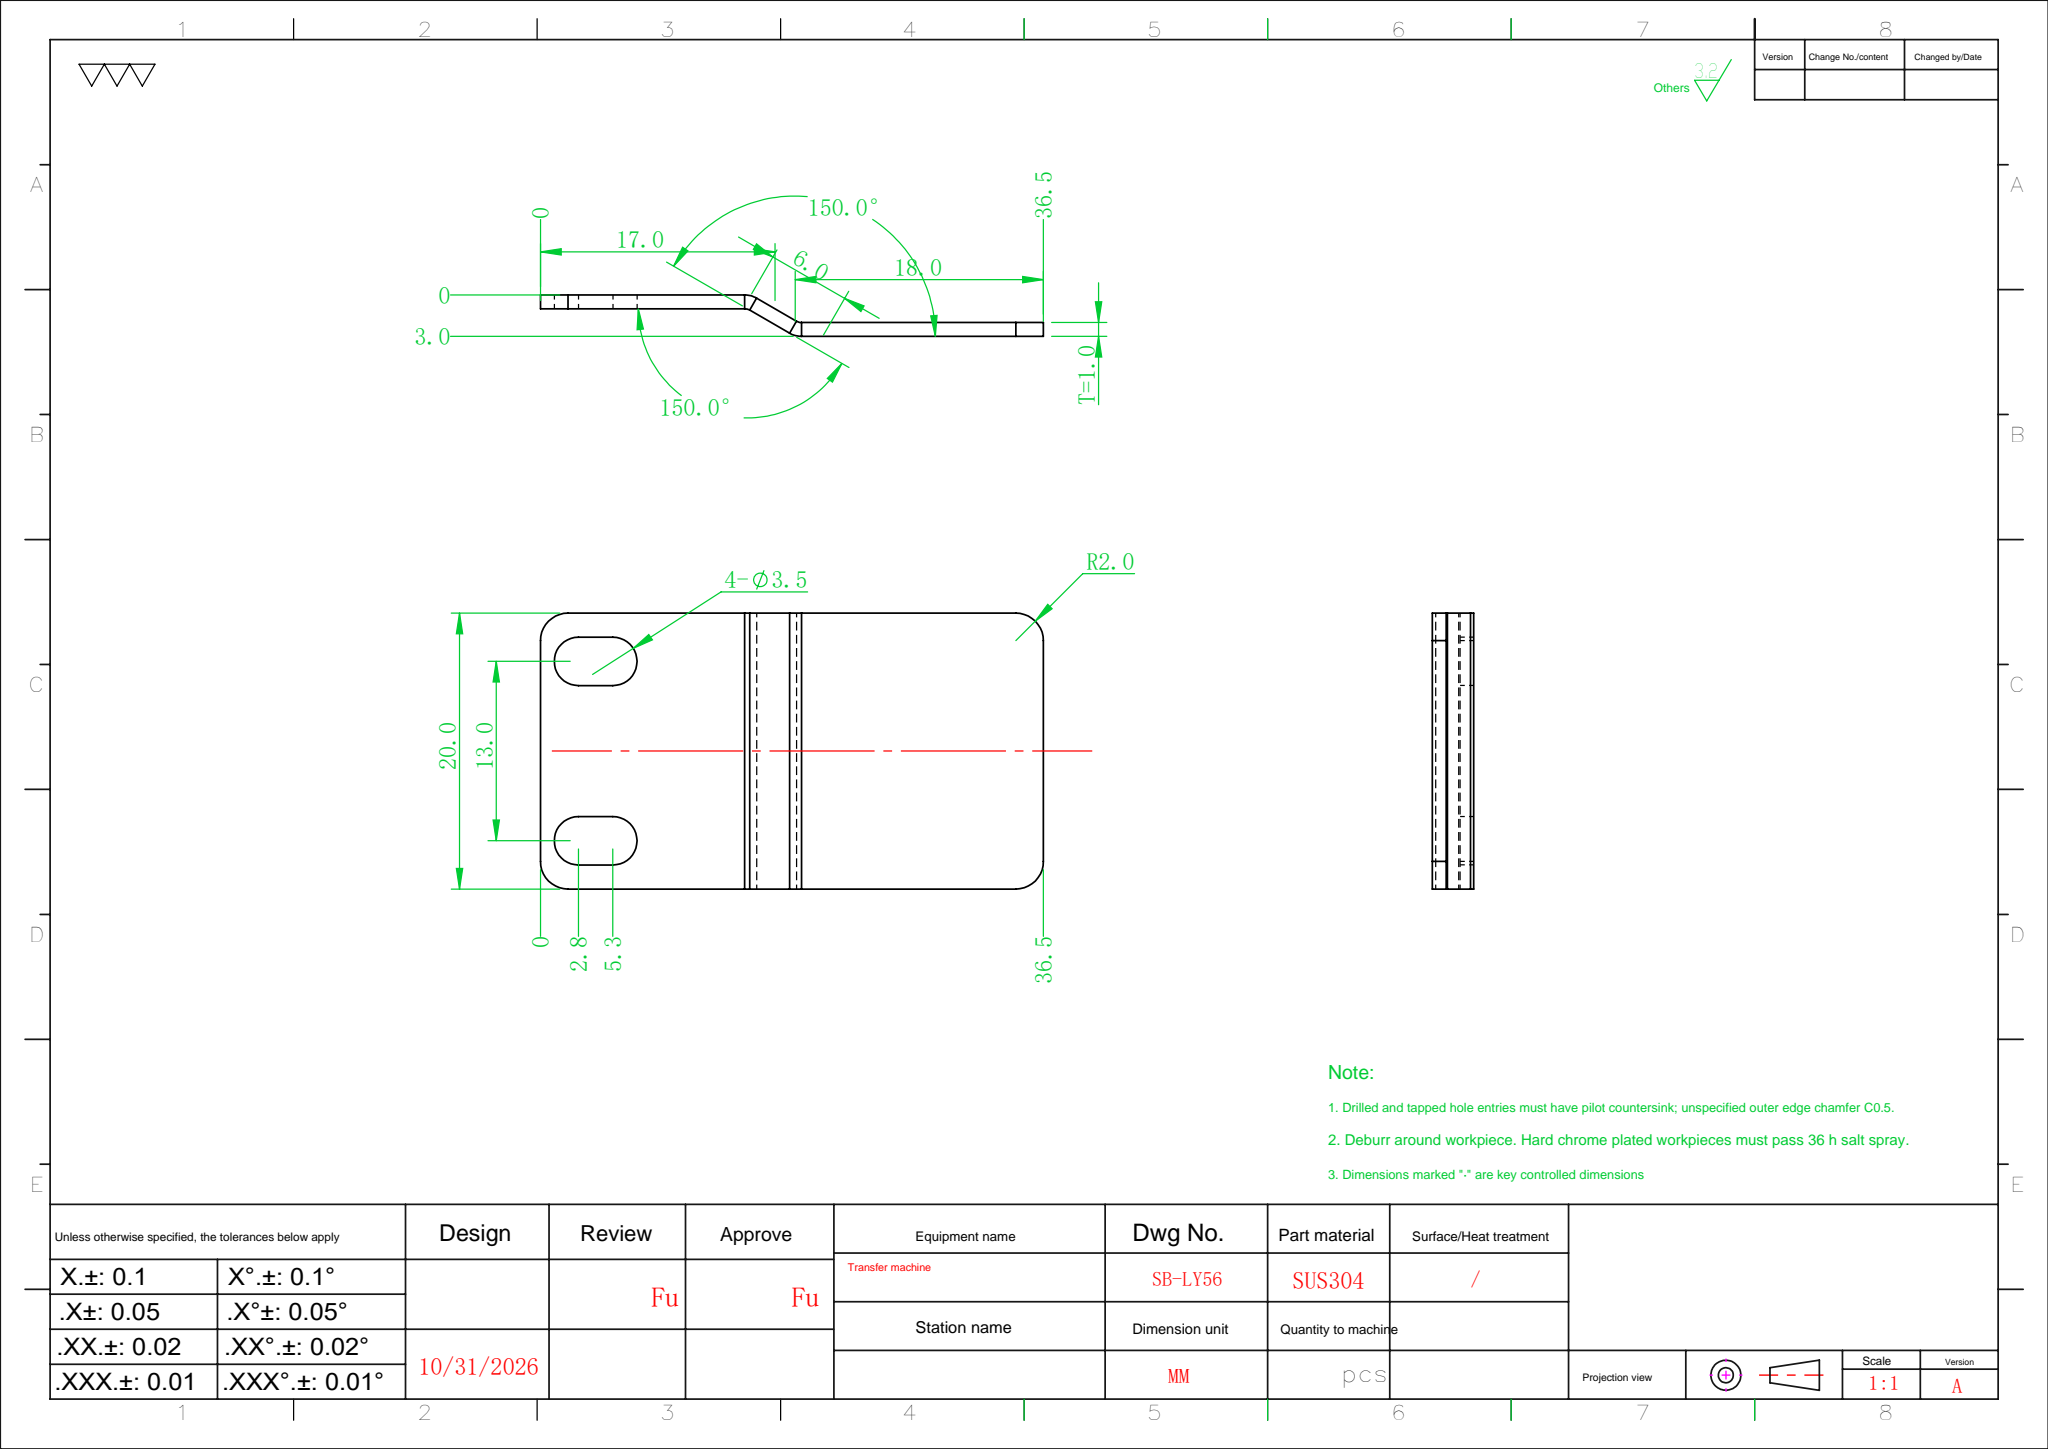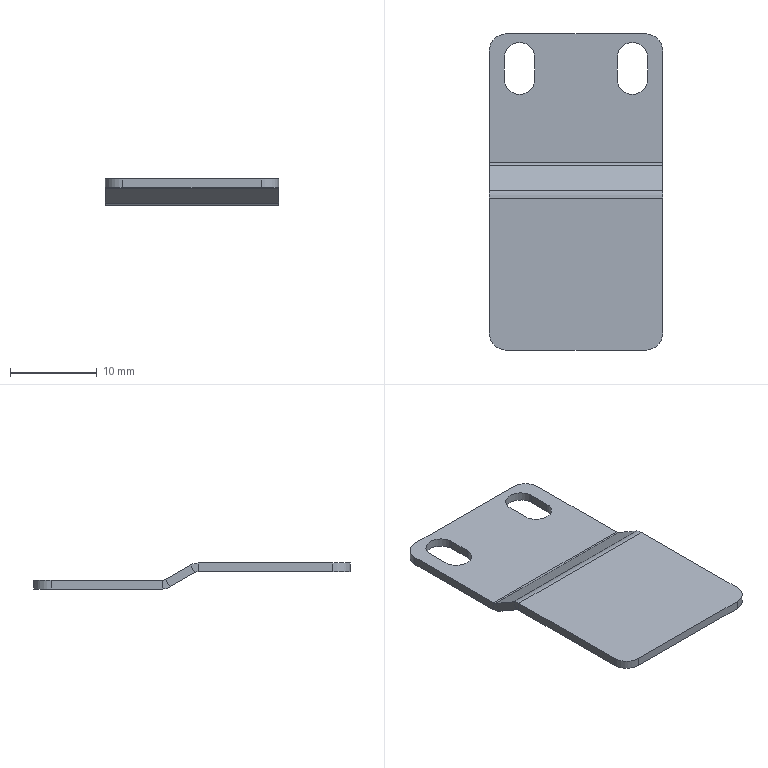Part | SolidWorks | features EdgeFlange 2, Fillet 1, FlatPattern 1, HoleWzd 1, SMBaseFlange 1, SheetMetal 1 | 1 solid | 34 faces | box 20 x 36.464 x 3 mm | volume 699.216 mm3 | plane 22 | cylinder 12 | commonest cylinder face diameters 3.5 x4 4 x4 1.473 x2 3.473 x2
STEP:
#1=CARTESIAN_POINT('',(-10.,-10.061,0.9013));
#2=VERTEX_POINT('',#1);
#3=CARTESIAN_POINT('',(-10.,-9.561,1.767));
#4=VERTEX_POINT('',#3);
#5=CARTESIAN_POINT('',(-10.,-10.061,0.9013));
#6=DIRECTION('',(0.,0.5,0.866));
#7=VECTOR('',#6,1000.);
#8=LINE('',#5,#7);
#9=EDGE_CURVE('',#2,#4,#8,.T.);
#10=ORIENTED_EDGE('',*,*,#9,.T.);
#11=CARTESIAN_POINT('',(-10.,-6.671,0.09869));
#12=VERTEX_POINT('',#11);
#13=CARTESIAN_POINT('',(-10.,-6.5,0.));
#14=DIRECTION('',(0.,0.866,-0.5));
#15=VECTOR('',#14,1000.);
#16=LINE('',#13,#15);
#17=EDGE_CURVE('',#4,#12,#16,.T.);
#18=ORIENTED_EDGE('',*,*,#17,.T.);
#19=CARTESIAN_POINT('',(-10.,-7.171,-0.7673));
#20=VERTEX_POINT('',#19);
#21=CARTESIAN_POINT('',(-10.,-7.171,-0.7673));
#22=DIRECTION('',(0.,-0.5,-0.866));
#23=VECTOR('',#22,1000.);
#24=LINE('',#21,#23);
#25=EDGE_CURVE('',#12,#20,#24,.T.);
#26=ORIENTED_EDGE('',*,*,#25,.T.);
#27=CARTESIAN_POINT('',(-10.,-0.625,-4.547));
#28=DIRECTION('',(0.,0.866,-0.5));
#29=VECTOR('',#28,1000.);
#30=LINE('',#27,#29);
#31=EDGE_CURVE('',#2,#20,#30,.T.);
#32=ORIENTED_EDGE('',*,*,#31,.F.);
#33=EDGE_LOOP('',(#10,#18,#26,#32));
#34=FACE_OUTER_BOUND('',#33,.T.);
#35=CARTESIAN_POINT('',(-10.,-7.,-0.866));
#36=DIRECTION('',(1.,0.,0.));
#37=DIRECTION('',(0.,1.,0.));
#38=AXIS2_PLACEMENT_3D('',#35,#36,#37);
#39=PLANE('',#38);
#40=ADVANCED_FACE('',(#34),#39,.F.);
#41=CARTESIAN_POINT('',(10.,-10.061,0.9013));
#42=VERTEX_POINT('',#41);
#43=CARTESIAN_POINT('',(10.,-9.561,1.767));
#44=VERTEX_POINT('',#43);
#45=CARTESIAN_POINT('',(10.,-10.061,0.9013));
#46=DIRECTION('',(0.,0.5,0.866));
#47=VECTOR('',#46,1000.);
#48=LINE('',#45,#47);
#49=EDGE_CURVE('',#42,#44,#48,.T.);
#50=ORIENTED_EDGE('',*,*,#49,.F.);
#51=CARTESIAN_POINT('',(10.,-7.171,-0.7673));
#52=VERTEX_POINT('',#51);
#53=CARTESIAN_POINT('',(10.,-0.625,-4.547));
#54=DIRECTION('',(0.,-0.866,0.5));
#55=VECTOR('',#54,1000.);
#56=LINE('',#53,#55);
#57=EDGE_CURVE('',#52,#42,#56,.T.);
#58=ORIENTED_EDGE('',*,*,#57,.F.);
#59=CARTESIAN_POINT('',(10.,-6.671,0.09869));
#60=VERTEX_POINT('',#59);
#61=CARTESIAN_POINT('',(10.,-6.671,0.09869));
#62=DIRECTION('',(0.,-0.5,-0.866));
#63=VECTOR('',#62,1000.);
#64=LINE('',#61,#63);
#65=EDGE_CURVE('',#60,#52,#64,.T.);
#66=ORIENTED_EDGE('',*,*,#65,.F.);
#67=CARTESIAN_POINT('',(10.,-11.464,2.866));
#68=DIRECTION('',(0.,-0.866,0.5));
#69=VECTOR('',#68,1000.);
#70=LINE('',#67,#69);
#71=EDGE_CURVE('',#60,#44,#70,.T.);
#72=ORIENTED_EDGE('',*,*,#71,.T.);
#73=EDGE_LOOP('',(#50,#58,#66,#72));
#74=FACE_OUTER_BOUND('',#73,.T.);
#75=CARTESIAN_POINT('',(10.,-11.964,2.));
#76=DIRECTION('',(-1.,0.,0.));
#77=DIRECTION('',(0.,-1.,0.));
#78=AXIS2_PLACEMENT_3D('',#75,#76,#77);
#79=PLANE('',#78);
#80=ADVANCED_FACE('',(#74),#79,.F.);
#81=CARTESIAN_POINT('',(-10.,-10.061,0.9013));
#82=DIRECTION('',(1.,0.,0.));
#83=VECTOR('',#82,1000.);
#84=LINE('',#81,#83);
#85=EDGE_CURVE('',#2,#42,#84,.T.);
#86=ORIENTED_EDGE('',*,*,#85,.F.);
#87=ORIENTED_EDGE('',*,*,#31,.T.);
#88=CARTESIAN_POINT('',(-10.,-7.171,-0.7673));
#89=DIRECTION('',(-1.,0.,0.));
#90=VECTOR('',#89,1000.);
#91=LINE('',#88,#90);
#92=EDGE_CURVE('',#52,#20,#91,.T.);
#93=ORIENTED_EDGE('',*,*,#92,.F.);
#94=ORIENTED_EDGE('',*,*,#57,.T.);
#95=EDGE_LOOP('',(#86,#87,#93,#94));
#96=FACE_OUTER_BOUND('',#95,.T.);
#97=CARTESIAN_POINT('',(0.,-0.625,-4.547));
#98=DIRECTION('',(0.,0.5,0.866));
#99=DIRECTION('',(0.,-0.866,0.5));
#100=AXIS2_PLACEMENT_3D('',#97,#98,#99);
#101=PLANE('',#100);
#102=ADVANCED_FACE('',(#96),#101,.F.);
#103=ORIENTED_EDGE('',*,*,#17,.F.);
#104=CARTESIAN_POINT('',(-10.,-9.561,1.767));
#105=DIRECTION('',(1.,0.,0.));
#106=VECTOR('',#105,1000.);
#107=LINE('',#104,#106);
#108=EDGE_CURVE('',#4,#44,#107,.T.);
#109=ORIENTED_EDGE('',*,*,#108,.T.);
#110=ORIENTED_EDGE('',*,*,#71,.F.);
#111=CARTESIAN_POINT('',(-10.,-6.671,0.09869));
#112=DIRECTION('',(1.,0.,0.));
#113=VECTOR('',#112,1000.);
#114=LINE('',#111,#113);
#115=EDGE_CURVE('',#12,#60,#114,.T.);
#116=ORIENTED_EDGE('',*,*,#115,.F.);
#117=EDGE_LOOP('',(#103,#109,#110,#116));
#118=FACE_OUTER_BOUND('',#117,.T.);
#119=CARTESIAN_POINT('',(0.,-0.125,-3.681));
#120=DIRECTION('',(0.,0.5,0.866));
#121=DIRECTION('',(0.,-0.866,0.5));
#122=AXIS2_PLACEMENT_3D('',#119,#120,#121);
#123=PLANE('',#122);
#124=ADVANCED_FACE('',(#118),#123,.T.);
#125=CARTESIAN_POINT('',(-4.75,5.75,0.));
#126=VERTEX_POINT('',#125);
#127=CARTESIAN_POINT('',(-8.25,5.75,0.));
#128=VERTEX_POINT('',#127);
#129=CARTESIAN_POINT('',(-6.5,5.75,0.));
#130=DIRECTION('',(0.,0.,1.));
#131=DIRECTION('',(1.,0.,0.));
#132=AXIS2_PLACEMENT_3D('',#129,#130,#131);
#133=CIRCLE('',#132,1.75);
#134=EDGE_CURVE('',#126,#128,#133,.T.);
#135=ORIENTED_EDGE('',*,*,#134,.F.);
#136=CARTESIAN_POINT('',(-4.75,3.25,0.));
#137=VERTEX_POINT('',#136);
#138=CARTESIAN_POINT('',(-4.75,3.25,0.));
#139=DIRECTION('',(0.,1.,0.));
#140=VECTOR('',#139,1000.);
#141=LINE('',#138,#140);
#142=EDGE_CURVE('',#137,#126,#141,.T.);
#143=ORIENTED_EDGE('',*,*,#142,.F.);
#144=CARTESIAN_POINT('',(-8.25,3.25,0.));
#145=VERTEX_POINT('',#144);
#146=CARTESIAN_POINT('',(-6.5,3.25,0.));
#147=DIRECTION('',(0.,0.,1.));
#148=DIRECTION('',(1.,0.,0.));
#149=AXIS2_PLACEMENT_3D('',#146,#147,#148);
#150=CIRCLE('',#149,1.75);
#151=EDGE_CURVE('',#145,#137,#150,.T.);
#152=ORIENTED_EDGE('',*,*,#151,.F.);
#153=CARTESIAN_POINT('',(-8.25,3.25,0.));
#154=DIRECTION('',(0.,1.,0.));
#155=VECTOR('',#154,1000.);
#156=LINE('',#153,#155);
#157=EDGE_CURVE('',#145,#128,#156,.T.);
#158=ORIENTED_EDGE('',*,*,#157,.T.);
#159=EDGE_LOOP('',(#135,#143,#152,#158));
#160=FACE_BOUND('',#159,.T.);
#161=CARTESIAN_POINT('',(8.25,5.75,0.));
#162=VERTEX_POINT('',#161);
#163=CARTESIAN_POINT('',(4.75,5.75,0.));
#164=VERTEX_POINT('',#163);
#165=CARTESIAN_POINT('',(6.5,5.75,0.));
#166=DIRECTION('',(0.,0.,1.));
#167=DIRECTION('',(1.,0.,0.));
#168=AXIS2_PLACEMENT_3D('',#165,#166,#167);
#169=CIRCLE('',#168,1.75);
#170=EDGE_CURVE('',#162,#164,#169,.T.);
#171=ORIENTED_EDGE('',*,*,#170,.F.);
#172=CARTESIAN_POINT('',(8.25,3.25,0.));
#173=VERTEX_POINT('',#172);
#174=CARTESIAN_POINT('',(8.25,3.25,0.));
#175=DIRECTION('',(0.,1.,0.));
#176=VECTOR('',#175,1000.);
#177=LINE('',#174,#176);
#178=EDGE_CURVE('',#173,#162,#177,.T.);
#179=ORIENTED_EDGE('',*,*,#178,.F.);
#180=CARTESIAN_POINT('',(4.75,3.25,0.));
#181=VERTEX_POINT('',#180);
#182=CARTESIAN_POINT('',(6.5,3.25,0.));
#183=DIRECTION('',(0.,0.,1.));
#184=DIRECTION('',(1.,0.,0.));
#185=AXIS2_PLACEMENT_3D('',#182,#183,#184);
#186=CIRCLE('',#185,1.75);
#187=EDGE_CURVE('',#181,#173,#186,.T.);
#188=ORIENTED_EDGE('',*,*,#187,.F.);
#189=CARTESIAN_POINT('',(4.75,3.25,0.));
#190=DIRECTION('',(0.,1.,0.));
#191=VECTOR('',#190,1000.);
#192=LINE('',#189,#191);
#193=EDGE_CURVE('',#181,#164,#192,.T.);
#194=ORIENTED_EDGE('',*,*,#193,.T.);
#195=EDGE_LOOP('',(#171,#179,#188,#194));
#196=FACE_BOUND('',#195,.T.);
#197=CARTESIAN_POINT('',(10.,-6.303,0.));
#198=VERTEX_POINT('',#197);
#199=CARTESIAN_POINT('',(10.,6.5,0.));
#200=VERTEX_POINT('',#199);
#201=CARTESIAN_POINT('',(10.,-8.5,0.));
#202=DIRECTION('',(0.,1.,0.));
#203=VECTOR('',#202,1000.);
#204=LINE('',#201,#203);
#205=EDGE_CURVE('',#198,#200,#204,.T.);
#206=ORIENTED_EDGE('',*,*,#205,.T.);
#207=CARTESIAN_POINT('',(8.,8.5,0.));
#208=VERTEX_POINT('',#207);
#209=CARTESIAN_POINT('',(8.,6.5,0.));
#210=DIRECTION('',(0.,0.,1.));
#211=DIRECTION('',(-1.,0.,0.));
#212=AXIS2_PLACEMENT_3D('',#209,#210,#211);
#213=CIRCLE('',#212,2.);
#214=EDGE_CURVE('',#200,#208,#213,.T.);
#215=ORIENTED_EDGE('',*,*,#214,.T.);
#216=CARTESIAN_POINT('',(-8.,8.5,0.));
#217=VERTEX_POINT('',#216);
#218=CARTESIAN_POINT('',(-10.,8.5,0.));
#219=DIRECTION('',(-1.,0.,0.));
#220=VECTOR('',#219,1000.);
#221=LINE('',#218,#220);
#222=EDGE_CURVE('',#208,#217,#221,.T.);
#223=ORIENTED_EDGE('',*,*,#222,.T.);
#224=CARTESIAN_POINT('',(-10.,6.5,0.));
#225=VERTEX_POINT('',#224);
#226=CARTESIAN_POINT('',(-8.,6.5,0.));
#227=DIRECTION('',(0.,0.,1.));
#228=DIRECTION('',(-1.,0.,0.));
#229=AXIS2_PLACEMENT_3D('',#226,#227,#228);
#230=CIRCLE('',#229,2.);
#231=EDGE_CURVE('',#217,#225,#230,.T.);
#232=ORIENTED_EDGE('',*,*,#231,.T.);
#233=CARTESIAN_POINT('',(-10.,-6.303,0.));
#234=VERTEX_POINT('',#233);
#235=CARTESIAN_POINT('',(-10.,-8.5,0.));
#236=DIRECTION('',(0.,-1.,0.));
#237=VECTOR('',#236,1000.);
#238=LINE('',#235,#237);
#239=EDGE_CURVE('',#225,#234,#238,.T.);
#240=ORIENTED_EDGE('',*,*,#239,.T.);
#241=CARTESIAN_POINT('',(10.,-6.303,0.));
#242=DIRECTION('',(-1.,0.,0.));
#243=VECTOR('',#242,1000.);
#244=LINE('',#241,#243);
#245=EDGE_CURVE('',#198,#234,#244,.T.);
#246=ORIENTED_EDGE('',*,*,#245,.F.);
#247=EDGE_LOOP('',(#206,#215,#223,#232,#240,#246));
#248=FACE_OUTER_BOUND('',#247,.T.);
#249=CARTESIAN_POINT('',(0.,0.,0.));
#250=DIRECTION('',(0.,0.,-1.));
#251=DIRECTION('',(-1.,0.,0.));
#252=AXIS2_PLACEMENT_3D('',#249,#250,#251);
#253=PLANE('',#252);
#254=ADVANCED_FACE('',(#160,#196,#248),#253,.F.);
#255=CARTESIAN_POINT('',(-4.75,5.75,-1.));
#256=VERTEX_POINT('',#255);
#257=CARTESIAN_POINT('',(-8.25,5.75,-1.));
#258=VERTEX_POINT('',#257);
#259=CARTESIAN_POINT('',(-6.5,5.75,-1.));
#260=DIRECTION('',(0.,0.,1.));
#261=DIRECTION('',(1.,0.,0.));
#262=AXIS2_PLACEMENT_3D('',#259,#260,#261);
#263=CIRCLE('',#262,1.75);
#264=EDGE_CURVE('',#256,#258,#263,.T.);
#265=ORIENTED_EDGE('',*,*,#264,.T.);
#266=CARTESIAN_POINT('',(-8.25,3.25,-1.));
#267=VERTEX_POINT('',#266);
#268=CARTESIAN_POINT('',(-8.25,3.25,-1.));
#269=DIRECTION('',(0.,1.,0.));
#270=VECTOR('',#269,1000.);
#271=LINE('',#268,#270);
#272=EDGE_CURVE('',#267,#258,#271,.T.);
#273=ORIENTED_EDGE('',*,*,#272,.F.);
#274=CARTESIAN_POINT('',(-4.75,3.25,-1.));
#275=VERTEX_POINT('',#274);
#276=CARTESIAN_POINT('',(-6.5,3.25,-1.));
#277=DIRECTION('',(0.,0.,1.));
#278=DIRECTION('',(1.,0.,0.));
#279=AXIS2_PLACEMENT_3D('',#276,#277,#278);
#280=CIRCLE('',#279,1.75);
#281=EDGE_CURVE('',#267,#275,#280,.T.);
#282=ORIENTED_EDGE('',*,*,#281,.T.);
#283=CARTESIAN_POINT('',(-4.75,3.25,-1.));
#284=DIRECTION('',(0.,1.,0.));
#285=VECTOR('',#284,1000.);
#286=LINE('',#283,#285);
#287=EDGE_CURVE('',#275,#256,#286,.T.);
#288=ORIENTED_EDGE('',*,*,#287,.T.);
#289=EDGE_LOOP('',(#265,#273,#282,#288));
#290=FACE_BOUND('',#289,.T.);
#291=CARTESIAN_POINT('',(4.75,3.25,-1.));
#292=VERTEX_POINT('',#291);
#293=CARTESIAN_POINT('',(8.25,3.25,-1.));
#294=VERTEX_POINT('',#293);
#295=CARTESIAN_POINT('',(6.5,3.25,-1.));
#296=DIRECTION('',(0.,0.,1.));
#297=DIRECTION('',(1.,0.,0.));
#298=AXIS2_PLACEMENT_3D('',#295,#296,#297);
#299=CIRCLE('',#298,1.75);
#300=EDGE_CURVE('',#292,#294,#299,.T.);
#301=ORIENTED_EDGE('',*,*,#300,.T.);
#302=CARTESIAN_POINT('',(8.25,5.75,-1.));
#303=VERTEX_POINT('',#302);
#304=CARTESIAN_POINT('',(8.25,3.25,-1.));
#305=DIRECTION('',(0.,1.,0.));
#306=VECTOR('',#305,1000.);
#307=LINE('',#304,#306);
#308=EDGE_CURVE('',#294,#303,#307,.T.);
#309=ORIENTED_EDGE('',*,*,#308,.T.);
#310=CARTESIAN_POINT('',(4.75,5.75,-1.));
#311=VERTEX_POINT('',#310);
#312=CARTESIAN_POINT('',(6.5,5.75,-1.));
#313=DIRECTION('',(0.,0.,1.));
#314=DIRECTION('',(1.,0.,0.));
#315=AXIS2_PLACEMENT_3D('',#312,#313,#314);
#316=CIRCLE('',#315,1.75);
#317=EDGE_CURVE('',#303,#311,#316,.T.);
#318=ORIENTED_EDGE('',*,*,#317,.T.);
#319=CARTESIAN_POINT('',(4.75,3.25,-1.));
#320=DIRECTION('',(0.,1.,0.));
#321=VECTOR('',#320,1000.);
#322=LINE('',#319,#321);
#323=EDGE_CURVE('',#292,#311,#322,.T.);
#324=ORIENTED_EDGE('',*,*,#323,.F.);
#325=EDGE_LOOP('',(#301,#309,#318,#324));
#326=FACE_BOUND('',#325,.T.);
#327=CARTESIAN_POINT('',(8.,8.5,-1.));
#328=VERTEX_POINT('',#327);
#329=CARTESIAN_POINT('',(-8.,8.5,-1.));
#330=VERTEX_POINT('',#329);
#331=CARTESIAN_POINT('',(-10.,8.5,-1.));
#332=DIRECTION('',(-1.,0.,0.));
#333=VECTOR('',#332,1000.);
#334=LINE('',#331,#333);
#335=EDGE_CURVE('',#328,#330,#334,.T.);
#336=ORIENTED_EDGE('',*,*,#335,.F.);
#337=CARTESIAN_POINT('',(10.,6.5,-1.));
#338=VERTEX_POINT('',#337);
#339=CARTESIAN_POINT('',(8.,6.5,-1.));
#340=DIRECTION('',(0.,0.,-1.));
#341=DIRECTION('',(-1.,0.,0.));
#342=AXIS2_PLACEMENT_3D('',#339,#340,#341);
#343=CIRCLE('',#342,2.);
#344=EDGE_CURVE('',#328,#338,#343,.T.);
#345=ORIENTED_EDGE('',*,*,#344,.T.);
#346=CARTESIAN_POINT('',(10.,-6.303,-1.));
#347=VERTEX_POINT('',#346);
#348=CARTESIAN_POINT('',(10.,-8.5,-1.));
#349=DIRECTION('',(0.,1.,0.));
#350=VECTOR('',#349,1000.);
#351=LINE('',#348,#350);
#352=EDGE_CURVE('',#347,#338,#351,.T.);
#353=ORIENTED_EDGE('',*,*,#352,.F.);
#354=CARTESIAN_POINT('',(-10.,-6.303,-1.));
#355=VERTEX_POINT('',#354);
#356=CARTESIAN_POINT('',(10.,-6.303,-1.));
#357=DIRECTION('',(-1.,0.,0.));
#358=VECTOR('',#357,1000.);
#359=LINE('',#356,#358);
#360=EDGE_CURVE('',#347,#355,#359,.T.);
#361=ORIENTED_EDGE('',*,*,#360,.T.);
#362=CARTESIAN_POINT('',(-10.,6.5,-1.));
#363=VERTEX_POINT('',#362);
#364=CARTESIAN_POINT('',(-10.,-8.5,-1.));
#365=DIRECTION('',(0.,-1.,0.));
#366=VECTOR('',#365,1000.);
#367=LINE('',#364,#366);
#368=EDGE_CURVE('',#363,#355,#367,.T.);
#369=ORIENTED_EDGE('',*,*,#368,.F.);
#370=CARTESIAN_POINT('',(-8.,6.5,-1.));
#371=DIRECTION('',(0.,0.,-1.));
#372=DIRECTION('',(-1.,0.,0.));
#373=AXIS2_PLACEMENT_3D('',#370,#371,#372);
#374=CIRCLE('',#373,2.);
#375=EDGE_CURVE('',#363,#330,#374,.T.);
#376=ORIENTED_EDGE('',*,*,#375,.T.);
#377=EDGE_LOOP('',(#336,#345,#353,#361,#369,#376));
#378=FACE_OUTER_BOUND('',#377,.T.);
#379=CARTESIAN_POINT('',(0.,0.,-1.));
#380=DIRECTION('',(0.,0.,-1.));
#381=DIRECTION('',(-1.,0.,0.));
#382=AXIS2_PLACEMENT_3D('',#379,#380,#381);
#383=PLANE('',#382);
#384=ADVANCED_FACE('',(#290,#326,#378),#383,.T.);
#385=ORIENTED_EDGE('',*,*,#352,.T.);
#386=CARTESIAN_POINT('',(10.,6.5,-1.));
#387=DIRECTION('',(0.,0.,1.));
#388=VECTOR('',#387,1000.);
#389=LINE('',#386,#388);
#390=EDGE_CURVE('',#338,#200,#389,.T.);
#391=ORIENTED_EDGE('',*,*,#390,.T.);
#392=ORIENTED_EDGE('',*,*,#205,.F.);
#393=CARTESIAN_POINT('',(10.,-6.303,0.));
#394=DIRECTION('',(0.,0.,-1.));
#395=VECTOR('',#394,1000.);
#396=LINE('',#393,#395);
#397=EDGE_CURVE('',#198,#347,#396,.T.);
#398=ORIENTED_EDGE('',*,*,#397,.T.);
#399=EDGE_LOOP('',(#385,#391,#392,#398));
#400=FACE_OUTER_BOUND('',#399,.T.);
#401=CARTESIAN_POINT('',(10.,-8.5,-1.));
#402=DIRECTION('',(1.,0.,0.));
#403=DIRECTION('',(0.,0.,-1.));
#404=AXIS2_PLACEMENT_3D('',#401,#402,#403);
#405=PLANE('',#404);
#406=ADVANCED_FACE('',(#400),#405,.T.);
#407=ORIENTED_EDGE('',*,*,#239,.F.);
#408=CARTESIAN_POINT('',(-10.,6.5,-1.));
#409=DIRECTION('',(0.,0.,-1.));
#410=VECTOR('',#409,1000.);
#411=LINE('',#408,#410);
#412=EDGE_CURVE('',#225,#363,#411,.T.);
#413=ORIENTED_EDGE('',*,*,#412,.T.);
#414=ORIENTED_EDGE('',*,*,#368,.T.);
#415=CARTESIAN_POINT('',(-10.,-6.303,0.));
#416=DIRECTION('',(0.,0.,-1.));
#417=VECTOR('',#416,1000.);
#418=LINE('',#415,#417);
#419=EDGE_CURVE('',#234,#355,#418,.T.);
#420=ORIENTED_EDGE('',*,*,#419,.F.);
#421=EDGE_LOOP('',(#407,#413,#414,#420));
#422=FACE_OUTER_BOUND('',#421,.T.);
#423=CARTESIAN_POINT('',(-10.,-8.5,-1.));
#424=DIRECTION('',(-1.,0.,0.));
#425=DIRECTION('',(0.,0.,1.));
#426=AXIS2_PLACEMENT_3D('',#423,#424,#425);
#427=PLANE('',#426);
#428=ADVANCED_FACE('',(#422),#427,.T.);
#429=ORIENTED_EDGE('',*,*,#222,.F.);
#430=CARTESIAN_POINT('',(8.,8.5,-1.));
#431=DIRECTION('',(0.,0.,-1.));
#432=VECTOR('',#431,1000.);
#433=LINE('',#430,#432);
#434=EDGE_CURVE('',#208,#328,#433,.T.);
#435=ORIENTED_EDGE('',*,*,#434,.T.);
#436=ORIENTED_EDGE('',*,*,#335,.T.);
#437=CARTESIAN_POINT('',(-8.,8.5,-1.));
#438=DIRECTION('',(0.,0.,1.));
#439=VECTOR('',#438,1000.);
#440=LINE('',#437,#439);
#441=EDGE_CURVE('',#330,#217,#440,.T.);
#442=ORIENTED_EDGE('',*,*,#441,.T.);
#443=EDGE_LOOP('',(#429,#435,#436,#442));
#444=FACE_OUTER_BOUND('',#443,.T.);
#445=CARTESIAN_POINT('',(-10.,8.5,-1.));
#446=DIRECTION('',(0.,1.,0.));
#447=DIRECTION('',(0.,0.,1.));
#448=AXIS2_PLACEMENT_3D('',#445,#446,#447);
#449=PLANE('',#448);
#450=ADVANCED_FACE('',(#444),#449,.T.);
#451=ORIENTED_EDGE('',*,*,#317,.F.);
#452=CARTESIAN_POINT('',(8.25,5.75,-1.));
#453=DIRECTION('',(0.,0.,-1.));
#454=VECTOR('',#453,1000.);
#455=LINE('',#452,#454);
#456=EDGE_CURVE('',#162,#303,#455,.T.);
#457=ORIENTED_EDGE('',*,*,#456,.F.);
#458=ORIENTED_EDGE('',*,*,#170,.T.);
#459=CARTESIAN_POINT('',(4.75,5.75,0.));
#460=DIRECTION('',(0.,0.,1.));
#461=VECTOR('',#460,1000.);
#462=LINE('',#459,#461);
#463=EDGE_CURVE('',#311,#164,#462,.T.);
#464=ORIENTED_EDGE('',*,*,#463,.F.);
#465=EDGE_LOOP('',(#451,#457,#458,#464));
#466=FACE_OUTER_BOUND('',#465,.T.);
#467=CARTESIAN_POINT('',(6.5,5.75,0.));
#468=DIRECTION('',(0.,0.,1.));
#469=DIRECTION('',(1.,0.,0.));
#470=AXIS2_PLACEMENT_3D('',#467,#468,#469);
#471=CYLINDRICAL_SURFACE('',#470,1.75);
#472=ADVANCED_FACE('',(#466),#471,.F.);
#473=ORIENTED_EDGE('',*,*,#187,.T.);
#474=CARTESIAN_POINT('',(8.25,3.25,-1.));
#475=DIRECTION('',(0.,0.,-1.));
#476=VECTOR('',#475,1000.);
#477=LINE('',#474,#476);
#478=EDGE_CURVE('',#173,#294,#477,.T.);
#479=ORIENTED_EDGE('',*,*,#478,.T.);
#480=ORIENTED_EDGE('',*,*,#300,.F.);
#481=CARTESIAN_POINT('',(4.75,3.25,0.));
#482=DIRECTION('',(0.,0.,-1.));
#483=VECTOR('',#482,1000.);
#484=LINE('',#481,#483);
#485=EDGE_CURVE('',#181,#292,#484,.T.);
#486=ORIENTED_EDGE('',*,*,#485,.F.);
#487=EDGE_LOOP('',(#473,#479,#480,#486));
#488=FACE_OUTER_BOUND('',#487,.T.);
#489=CARTESIAN_POINT('',(6.5,3.25,0.));
#490=DIRECTION('',(0.,0.,1.));
#491=DIRECTION('',(1.,0.,0.));
#492=AXIS2_PLACEMENT_3D('',#489,#490,#491);
#493=CYLINDRICAL_SURFACE('',#492,1.75);
#494=ADVANCED_FACE('',(#488),#493,.F.);
#495=ORIENTED_EDGE('',*,*,#463,.T.);
#496=ORIENTED_EDGE('',*,*,#193,.F.);
#497=ORIENTED_EDGE('',*,*,#485,.T.);
#498=ORIENTED_EDGE('',*,*,#323,.T.);
#499=EDGE_LOOP('',(#495,#496,#497,#498));
#500=FACE_OUTER_BOUND('',#499,.T.);
#501=CARTESIAN_POINT('',(4.75,3.25,0.));
#502=DIRECTION('',(-1.,0.,0.));
#503=DIRECTION('',(0.,0.,1.));
#504=AXIS2_PLACEMENT_3D('',#501,#502,#503);
#505=PLANE('',#504);
#506=ADVANCED_FACE('',(#500),#505,.F.);
#507=ORIENTED_EDGE('',*,*,#456,.T.);
#508=ORIENTED_EDGE('',*,*,#308,.F.);
#509=ORIENTED_EDGE('',*,*,#478,.F.);
#510=ORIENTED_EDGE('',*,*,#178,.T.);
#511=EDGE_LOOP('',(#507,#508,#509,#510));
#512=FACE_OUTER_BOUND('',#511,.T.);
#513=CARTESIAN_POINT('',(8.25,3.25,-1.));
#514=DIRECTION('',(1.,0.,0.));
#515=DIRECTION('',(0.,0.,-1.));
#516=AXIS2_PLACEMENT_3D('',#513,#514,#515);
#517=PLANE('',#516);
#518=ADVANCED_FACE('',(#512),#517,.F.);
#519=ORIENTED_EDGE('',*,*,#264,.F.);
#520=CARTESIAN_POINT('',(-4.75,5.75,-1.));
#521=DIRECTION('',(0.,0.,-1.));
#522=VECTOR('',#521,1000.);
#523=LINE('',#520,#522);
#524=EDGE_CURVE('',#126,#256,#523,.T.);
#525=ORIENTED_EDGE('',*,*,#524,.F.);
#526=ORIENTED_EDGE('',*,*,#134,.T.);
#527=CARTESIAN_POINT('',(-8.25,5.75,0.));
#528=DIRECTION('',(0.,0.,1.));
#529=VECTOR('',#528,1000.);
#530=LINE('',#527,#529);
#531=EDGE_CURVE('',#258,#128,#530,.T.);
#532=ORIENTED_EDGE('',*,*,#531,.F.);
#533=EDGE_LOOP('',(#519,#525,#526,#532));
#534=FACE_OUTER_BOUND('',#533,.T.);
#535=CARTESIAN_POINT('',(-6.5,5.75,0.));
#536=DIRECTION('',(0.,0.,1.));
#537=DIRECTION('',(1.,0.,0.));
#538=AXIS2_PLACEMENT_3D('',#535,#536,#537);
#539=CYLINDRICAL_SURFACE('',#538,1.75);
#540=ADVANCED_FACE('',(#534),#539,.F.);
#541=ORIENTED_EDGE('',*,*,#151,.T.);
#542=CARTESIAN_POINT('',(-4.75,3.25,-1.));
#543=DIRECTION('',(0.,0.,-1.));
#544=VECTOR('',#543,1000.);
#545=LINE('',#542,#544);
#546=EDGE_CURVE('',#137,#275,#545,.T.);
#547=ORIENTED_EDGE('',*,*,#546,.T.);
#548=ORIENTED_EDGE('',*,*,#281,.F.);
#549=CARTESIAN_POINT('',(-8.25,3.25,0.));
#550=DIRECTION('',(0.,0.,-1.));
#551=VECTOR('',#550,1000.);
#552=LINE('',#549,#551);
#553=EDGE_CURVE('',#145,#267,#552,.T.);
#554=ORIENTED_EDGE('',*,*,#553,.F.);
#555=EDGE_LOOP('',(#541,#547,#548,#554));
#556=FACE_OUTER_BOUND('',#555,.T.);
#557=CARTESIAN_POINT('',(-6.5,3.25,0.));
#558=DIRECTION('',(0.,0.,1.));
#559=DIRECTION('',(1.,0.,0.));
#560=AXIS2_PLACEMENT_3D('',#557,#558,#559);
#561=CYLINDRICAL_SURFACE('',#560,1.75);
#562=ADVANCED_FACE('',(#556),#561,.F.);
#563=ORIENTED_EDGE('',*,*,#531,.T.);
#564=ORIENTED_EDGE('',*,*,#157,.F.);
#565=ORIENTED_EDGE('',*,*,#553,.T.);
#566=ORIENTED_EDGE('',*,*,#272,.T.);
#567=EDGE_LOOP('',(#563,#564,#565,#566));
#568=FACE_OUTER_BOUND('',#567,.T.);
#569=CARTESIAN_POINT('',(-8.25,3.25,0.));
#570=DIRECTION('',(-1.,0.,0.));
#571=DIRECTION('',(0.,0.,1.));
#572=AXIS2_PLACEMENT_3D('',#569,#570,#571);
#573=PLANE('',#572);
#574=ADVANCED_FACE('',(#568),#573,.F.);
#575=ORIENTED_EDGE('',*,*,#524,.T.);
#576=ORIENTED_EDGE('',*,*,#287,.F.);
#577=ORIENTED_EDGE('',*,*,#546,.F.);
#578=ORIENTED_EDGE('',*,*,#142,.T.);
#579=EDGE_LOOP('',(#575,#576,#577,#578));
#580=FACE_OUTER_BOUND('',#579,.T.);
#581=CARTESIAN_POINT('',(-4.75,3.25,-1.));
#582=DIRECTION('',(1.,0.,0.));
#583=DIRECTION('',(0.,0.,-1.));
#584=AXIS2_PLACEMENT_3D('',#581,#582,#583);
#585=PLANE('',#584);
#586=ADVANCED_FACE('',(#580),#585,.F.);
#587=ORIENTED_EDGE('',*,*,#25,.F.);
#588=CARTESIAN_POINT('',(-10.,-6.303,0.7366));
#589=DIRECTION('',(-1.,0.,0.));
#590=DIRECTION('',(0.,0.,-1.));
#591=AXIS2_PLACEMENT_3D('',#588,#589,#590);
#592=CIRCLE('',#591,0.7366);
#593=EDGE_CURVE('',#234,#12,#592,.T.);
#594=ORIENTED_EDGE('',*,*,#593,.F.);
#595=ORIENTED_EDGE('',*,*,#419,.T.);
#596=CARTESIAN_POINT('',(-10.,-6.303,0.7366));
#597=DIRECTION('',(-1.,0.,0.));
#598=DIRECTION('',(0.,0.,-1.));
#599=AXIS2_PLACEMENT_3D('',#596,#597,#598);
#600=CIRCLE('',#599,1.737);
#601=EDGE_CURVE('',#355,#20,#600,.T.);
#602=ORIENTED_EDGE('',*,*,#601,.T.);
#603=EDGE_LOOP('',(#587,#594,#595,#602));
#604=FACE_OUTER_BOUND('',#603,.T.);
#605=CARTESIAN_POINT('',(-10.,-6.303,0.7366));
#606=DIRECTION('',(-1.,0.,0.));
#607=DIRECTION('',(0.,0.,1.));
#608=AXIS2_PLACEMENT_3D('',#605,#606,#607);
#609=PLANE('',#608);
#610=ADVANCED_FACE('',(#604),#609,.T.);
#611=CARTESIAN_POINT('',(10.,-6.303,0.7366));
#612=DIRECTION('',(1.,0.,0.));
#613=DIRECTION('',(0.,0.,-1.));
#614=AXIS2_PLACEMENT_3D('',#611,#612,#613);
#615=CIRCLE('',#614,0.7366);
#616=EDGE_CURVE('',#60,#198,#615,.T.);
#617=ORIENTED_EDGE('',*,*,#616,.F.);
#618=ORIENTED_EDGE('',*,*,#65,.T.);
#619=CARTESIAN_POINT('',(10.,-6.303,0.7366));
#620=DIRECTION('',(1.,0.,0.));
#621=DIRECTION('',(0.,0.,-1.));
#622=AXIS2_PLACEMENT_3D('',#619,#620,#621);
#623=CIRCLE('',#622,1.737);
#624=EDGE_CURVE('',#52,#347,#623,.T.);
#625=ORIENTED_EDGE('',*,*,#624,.T.);
#626=ORIENTED_EDGE('',*,*,#397,.F.);
#627=EDGE_LOOP('',(#617,#618,#625,#626));
#628=FACE_OUTER_BOUND('',#627,.T.);
#629=CARTESIAN_POINT('',(10.,-6.303,0.7366));
#630=DIRECTION('',(-1.,0.,0.));
#631=DIRECTION('',(0.,0.,1.));
#632=AXIS2_PLACEMENT_3D('',#629,#630,#631);
#633=PLANE('',#632);
#634=ADVANCED_FACE('',(#628),#633,.F.);
#635=ORIENTED_EDGE('',*,*,#360,.F.);
#636=ORIENTED_EDGE('',*,*,#624,.F.);
#637=ORIENTED_EDGE('',*,*,#92,.T.);
#638=ORIENTED_EDGE('',*,*,#601,.F.);
#639=EDGE_LOOP('',(#635,#636,#637,#638));
#640=FACE_OUTER_BOUND('',#639,.T.);
#641=CARTESIAN_POINT('',(10.,-6.303,0.7366));
#642=DIRECTION('',(1.,0.,0.));
#643=DIRECTION('',(0.,-0.5,-0.866));
#644=AXIS2_PLACEMENT_3D('',#641,#642,#643);
#645=CYLINDRICAL_SURFACE('',#644,1.737);
#646=ADVANCED_FACE('',(#640),#645,.T.);
#647=ORIENTED_EDGE('',*,*,#245,.T.);
#648=ORIENTED_EDGE('',*,*,#593,.T.);
#649=ORIENTED_EDGE('',*,*,#115,.T.);
#650=ORIENTED_EDGE('',*,*,#616,.T.);
#651=EDGE_LOOP('',(#647,#648,#649,#650));
#652=FACE_OUTER_BOUND('',#651,.T.);
#653=CARTESIAN_POINT('',(10.,-6.303,0.7366));
#654=DIRECTION('',(1.,0.,0.));
#655=DIRECTION('',(0.,-0.5,-0.866));
#656=AXIS2_PLACEMENT_3D('',#653,#654,#655);
#657=CYLINDRICAL_SURFACE('',#656,0.7366);
#658=ADVANCED_FACE('',(#652),#657,.F.);
#659=CARTESIAN_POINT('',(10.,-10.429,1.));
#660=VERTEX_POINT('',#659);
#661=CARTESIAN_POINT('',(10.,-10.429,2.));
#662=VERTEX_POINT('',#661);
#663=CARTESIAN_POINT('',(10.,-10.429,2.));
#664=DIRECTION('',(0.,0.,1.));
#665=VECTOR('',#664,1000.);
#666=LINE('',#663,#665);
#667=EDGE_CURVE('',#660,#662,#666,.T.);
#668=ORIENTED_EDGE('',*,*,#667,.F.);
#669=CARTESIAN_POINT('',(10.,-10.429,0.2634));
#670=DIRECTION('',(1.,0.,0.));
#671=DIRECTION('',(0.,0.,1.));
#672=AXIS2_PLACEMENT_3D('',#669,#670,#671);
#673=CIRCLE('',#672,0.7366);
#674=EDGE_CURVE('',#42,#660,#673,.T.);
#675=ORIENTED_EDGE('',*,*,#674,.F.);
#676=ORIENTED_EDGE('',*,*,#49,.T.);
#677=CARTESIAN_POINT('',(10.,-10.429,0.2634));
#678=DIRECTION('',(1.,0.,0.));
#679=DIRECTION('',(0.,0.,1.));
#680=AXIS2_PLACEMENT_3D('',#677,#678,#679);
#681=CIRCLE('',#680,1.737);
#682=EDGE_CURVE('',#44,#662,#681,.T.);
#683=ORIENTED_EDGE('',*,*,#682,.T.);
#684=EDGE_LOOP('',(#668,#675,#676,#683));
#685=FACE_OUTER_BOUND('',#684,.T.);
#686=CARTESIAN_POINT('',(10.,-10.429,0.2634));
#687=DIRECTION('',(1.,0.,0.));
#688=DIRECTION('',(0.,0.,-1.));
#689=AXIS2_PLACEMENT_3D('',#686,#687,#688);
#690=PLANE('',#689);
#691=ADVANCED_FACE('',(#685),#690,.T.);
#692=CARTESIAN_POINT('',(-10.,-10.429,1.));
#693=VERTEX_POINT('',#692);
#694=CARTESIAN_POINT('',(-10.,-10.429,0.2634));
#695=DIRECTION('',(-1.,0.,0.));
#696=DIRECTION('',(0.,0.,1.));
#697=AXIS2_PLACEMENT_3D('',#694,#695,#696);
#698=CIRCLE('',#697,0.7366);
#699=EDGE_CURVE('',#693,#2,#698,.T.);
#700=ORIENTED_EDGE('',*,*,#699,.F.);
#701=CARTESIAN_POINT('',(-10.,-10.429,2.));
#702=VERTEX_POINT('',#701);
#703=CARTESIAN_POINT('',(-10.,-10.429,1.));
#704=DIRECTION('',(0.,0.,1.));
#705=VECTOR('',#704,1000.);
#706=LINE('',#703,#705);
#707=EDGE_CURVE('',#693,#702,#706,.T.);
#708=ORIENTED_EDGE('',*,*,#707,.T.);
#709=CARTESIAN_POINT('',(-10.,-10.429,0.2634));
#710=DIRECTION('',(-1.,0.,0.));
#711=DIRECTION('',(0.,0.,1.));
#712=AXIS2_PLACEMENT_3D('',#709,#710,#711);
#713=CIRCLE('',#712,1.737);
#714=EDGE_CURVE('',#702,#4,#713,.T.);
#715=ORIENTED_EDGE('',*,*,#714,.T.);
#716=ORIENTED_EDGE('',*,*,#9,.F.);
#717=EDGE_LOOP('',(#700,#708,#715,#716));
#718=FACE_OUTER_BOUND('',#717,.T.);
#719=CARTESIAN_POINT('',(-10.,-10.429,0.2634));
#720=DIRECTION('',(1.,0.,0.));
#721=DIRECTION('',(0.,0.,-1.));
#722=AXIS2_PLACEMENT_3D('',#719,#720,#721);
#723=PLANE('',#722);
#724=ADVANCED_FACE('',(#718),#723,.F.);
#725=ORIENTED_EDGE('',*,*,#108,.F.);
#726=ORIENTED_EDGE('',*,*,#714,.F.);
#727=CARTESIAN_POINT('',(0.,-10.429,2.));
#728=DIRECTION('',(-1.,0.,0.));
#729=VECTOR('',#728,1000.);
#730=LINE('',#727,#729);
#731=EDGE_CURVE('',#662,#702,#730,.T.);
#732=ORIENTED_EDGE('',*,*,#731,.F.);
#733=ORIENTED_EDGE('',*,*,#682,.F.);
#734=EDGE_LOOP('',(#725,#726,#732,#733));
#735=FACE_OUTER_BOUND('',#734,.T.);
#736=CARTESIAN_POINT('',(-10.,-10.429,0.2634));
#737=DIRECTION('',(-1.,0.,0.));
#738=DIRECTION('',(0.,0.,1.));
#739=AXIS2_PLACEMENT_3D('',#736,#737,#738);
#740=CYLINDRICAL_SURFACE('',#739,1.737);
#741=ADVANCED_FACE('',(#735),#740,.T.);
#742=ORIENTED_EDGE('',*,*,#85,.T.);
#743=ORIENTED_EDGE('',*,*,#674,.T.);
#744=CARTESIAN_POINT('',(10.,-10.429,1.));
#745=DIRECTION('',(-1.,0.,0.));
#746=VECTOR('',#745,1000.);
#747=LINE('',#744,#746);
#748=EDGE_CURVE('',#660,#693,#747,.T.);
#749=ORIENTED_EDGE('',*,*,#748,.T.);
#750=ORIENTED_EDGE('',*,*,#699,.T.);
#751=EDGE_LOOP('',(#742,#743,#749,#750));
#752=FACE_OUTER_BOUND('',#751,.T.);
#753=CARTESIAN_POINT('',(-10.,-10.429,0.2634));
#754=DIRECTION('',(-1.,0.,0.));
#755=DIRECTION('',(0.,0.,1.));
#756=AXIS2_PLACEMENT_3D('',#753,#754,#755);
#757=CYLINDRICAL_SURFACE('',#756,0.7366);
#758=ADVANCED_FACE('',(#752),#757,.F.);
#759=CARTESIAN_POINT('',(-10.,-25.964,1.));
#760=VERTEX_POINT('',#759);
#761=CARTESIAN_POINT('',(-10.,1.732,1.));
#762=DIRECTION('',(0.,1.,0.));
#763=VECTOR('',#762,1000.);
#764=LINE('',#761,#763);
#765=EDGE_CURVE('',#760,#693,#764,.T.);
#766=ORIENTED_EDGE('',*,*,#765,.F.);
#767=CARTESIAN_POINT('',(-10.,-25.964,2.));
#768=VERTEX_POINT('',#767);
#769=CARTESIAN_POINT('',(-10.,-25.964,2.));
#770=DIRECTION('',(0.,0.,1.));
#771=VECTOR('',#770,1000.);
#772=LINE('',#769,#771);
#773=EDGE_CURVE('',#760,#768,#772,.T.);
#774=ORIENTED_EDGE('',*,*,#773,.T.);
#775=CARTESIAN_POINT('',(-10.,-10.232,2.));
#776=DIRECTION('',(0.,1.,0.));
#777=VECTOR('',#776,1000.);
#778=LINE('',#775,#777);
#779=EDGE_CURVE('',#768,#702,#778,.T.);
#780=ORIENTED_EDGE('',*,*,#779,.T.);
#781=ORIENTED_EDGE('',*,*,#707,.F.);
#782=EDGE_LOOP('',(#766,#774,#780,#781));
#783=FACE_OUTER_BOUND('',#782,.T.);
#784=CARTESIAN_POINT('',(-10.,-10.232,2.));
#785=DIRECTION('',(-1.,0.,0.));
#786=DIRECTION('',(0.,-1.,0.));
#787=AXIS2_PLACEMENT_3D('',#784,#785,#786);
#788=PLANE('',#787);
#789=ADVANCED_FACE('',(#783),#788,.T.);
#790=CARTESIAN_POINT('',(10.,-25.964,2.));
#791=VERTEX_POINT('',#790);
#792=CARTESIAN_POINT('',(10.,-27.964,2.));
#793=DIRECTION('',(0.,-1.,0.));
#794=VECTOR('',#793,1000.);
#795=LINE('',#792,#794);
#796=EDGE_CURVE('',#662,#791,#795,.T.);
#797=ORIENTED_EDGE('',*,*,#796,.T.);
#798=CARTESIAN_POINT('',(10.,-25.964,1.));
#799=VERTEX_POINT('',#798);
#800=CARTESIAN_POINT('',(10.,-25.964,2.));
#801=DIRECTION('',(0.,0.,-1.));
#802=VECTOR('',#801,1000.);
#803=LINE('',#800,#802);
#804=EDGE_CURVE('',#791,#799,#803,.T.);
#805=ORIENTED_EDGE('',*,*,#804,.T.);
#806=CARTESIAN_POINT('',(10.,1.732,1.));
#807=DIRECTION('',(0.,-1.,0.));
#808=VECTOR('',#807,1000.);
#809=LINE('',#806,#808);
#810=EDGE_CURVE('',#660,#799,#809,.T.);
#811=ORIENTED_EDGE('',*,*,#810,.F.);
#812=ORIENTED_EDGE('',*,*,#667,.T.);
#813=EDGE_LOOP('',(#797,#805,#811,#812));
#814=FACE_OUTER_BOUND('',#813,.T.);
#815=CARTESIAN_POINT('',(10.,-27.964,2.));
#816=DIRECTION('',(1.,0.,0.));
#817=DIRECTION('',(0.,1.,0.));
#818=AXIS2_PLACEMENT_3D('',#815,#816,#817);
#819=PLANE('',#818);
#820=ADVANCED_FACE('',(#814),#819,.T.);
#821=ORIENTED_EDGE('',*,*,#779,.F.);
#822=CARTESIAN_POINT('',(-8.,-27.964,2.));
#823=VERTEX_POINT('',#822);
#824=CARTESIAN_POINT('',(-8.,-25.964,2.));
#825=DIRECTION('',(0.,0.,1.));
#826=DIRECTION('',(1.,0.,0.));
#827=AXIS2_PLACEMENT_3D('',#824,#825,#826);
#828=CIRCLE('',#827,2.);
#829=EDGE_CURVE('',#768,#823,#828,.T.);
#830=ORIENTED_EDGE('',*,*,#829,.T.);
#831=CARTESIAN_POINT('',(8.,-27.964,2.));
#832=VERTEX_POINT('',#831);
#833=CARTESIAN_POINT('',(-10.,-27.964,2.));
#834=DIRECTION('',(-1.,0.,0.));
#835=VECTOR('',#834,1000.);
#836=LINE('',#833,#835);
#837=EDGE_CURVE('',#832,#823,#836,.T.);
#838=ORIENTED_EDGE('',*,*,#837,.F.);
#839=CARTESIAN_POINT('',(8.,-25.964,2.));
#840=DIRECTION('',(0.,0.,1.));
#841=DIRECTION('',(1.,0.,0.));
#842=AXIS2_PLACEMENT_3D('',#839,#840,#841);
#843=CIRCLE('',#842,2.);
#844=EDGE_CURVE('',#832,#791,#843,.T.);
#845=ORIENTED_EDGE('',*,*,#844,.T.);
#846=ORIENTED_EDGE('',*,*,#796,.F.);
#847=ORIENTED_EDGE('',*,*,#731,.T.);
#848=EDGE_LOOP('',(#821,#830,#838,#845,#846,#847));
#849=FACE_OUTER_BOUND('',#848,.T.);
#850=CARTESIAN_POINT('',(0.,1.732,2.));
#851=DIRECTION('',(0.,0.,1.));
#852=DIRECTION('',(1.,0.,0.));
#853=AXIS2_PLACEMENT_3D('',#850,#851,#852);
#854=PLANE('',#853);
#855=ADVANCED_FACE('',(#849),#854,.T.);
#856=CARTESIAN_POINT('',(8.,-27.964,1.));
#857=VERTEX_POINT('',#856);
#858=CARTESIAN_POINT('',(-8.,-27.964,1.));
#859=VERTEX_POINT('',#858);
#860=CARTESIAN_POINT('',(0.,-27.964,1.));
#861=DIRECTION('',(-1.,0.,0.));
#862=VECTOR('',#861,1000.);
#863=LINE('',#860,#862);
#864=EDGE_CURVE('',#857,#859,#863,.T.);
#865=ORIENTED_EDGE('',*,*,#864,.T.);
#866=CARTESIAN_POINT('',(-8.,-25.964,1.));
#867=DIRECTION('',(0.,0.,-1.));
#868=DIRECTION('',(1.,0.,0.));
#869=AXIS2_PLACEMENT_3D('',#866,#867,#868);
#870=CIRCLE('',#869,2.);
#871=EDGE_CURVE('',#859,#760,#870,.T.);
#872=ORIENTED_EDGE('',*,*,#871,.T.);
#873=ORIENTED_EDGE('',*,*,#765,.T.);
#874=ORIENTED_EDGE('',*,*,#748,.F.);
#875=ORIENTED_EDGE('',*,*,#810,.T.);
#876=CARTESIAN_POINT('',(8.,-25.964,1.));
#877=DIRECTION('',(0.,0.,-1.));
#878=DIRECTION('',(1.,0.,0.));
#879=AXIS2_PLACEMENT_3D('',#876,#877,#878);
#880=CIRCLE('',#879,2.);
#881=EDGE_CURVE('',#799,#857,#880,.T.);
#882=ORIENTED_EDGE('',*,*,#881,.T.);
#883=EDGE_LOOP('',(#865,#872,#873,#874,#875,#882));
#884=FACE_OUTER_BOUND('',#883,.T.);
#885=CARTESIAN_POINT('',(0.,1.732,1.));
#886=DIRECTION('',(0.,0.,1.));
#887=DIRECTION('',(1.,0.,0.));
#888=AXIS2_PLACEMENT_3D('',#885,#886,#887);
#889=PLANE('',#888);
#890=ADVANCED_FACE('',(#884),#889,.F.);
#891=ORIENTED_EDGE('',*,*,#837,.T.);
#892=CARTESIAN_POINT('',(-8.,-27.964,2.));
#893=DIRECTION('',(0.,0.,-1.));
#894=VECTOR('',#893,1000.);
#895=LINE('',#892,#894);
#896=EDGE_CURVE('',#823,#859,#895,.T.);
#897=ORIENTED_EDGE('',*,*,#896,.T.);
#898=ORIENTED_EDGE('',*,*,#864,.F.);
#899=CARTESIAN_POINT('',(8.,-27.964,2.));
#900=DIRECTION('',(0.,0.,1.));
#901=VECTOR('',#900,1000.);
#902=LINE('',#899,#901);
#903=EDGE_CURVE('',#857,#832,#902,.T.);
#904=ORIENTED_EDGE('',*,*,#903,.T.);
#905=EDGE_LOOP('',(#891,#897,#898,#904));
#906=FACE_OUTER_BOUND('',#905,.T.);
#907=CARTESIAN_POINT('',(-10.,-27.964,2.));
#908=DIRECTION('',(0.,-1.,0.));
#909=DIRECTION('',(0.,0.,-1.));
#910=AXIS2_PLACEMENT_3D('',#907,#908,#909);
#911=PLANE('',#910);
#912=ADVANCED_FACE('',(#906),#911,.T.);
#913=ORIENTED_EDGE('',*,*,#829,.F.);
#914=ORIENTED_EDGE('',*,*,#773,.F.);
#915=ORIENTED_EDGE('',*,*,#871,.F.);
#916=ORIENTED_EDGE('',*,*,#896,.F.);
#917=EDGE_LOOP('',(#913,#914,#915,#916));
#918=FACE_OUTER_BOUND('',#917,.T.);
#919=CARTESIAN_POINT('',(-8.,-25.964,2.));
#920=DIRECTION('',(0.,0.,-1.));
#921=DIRECTION('',(-1.,0.,0.));
#922=AXIS2_PLACEMENT_3D('',#919,#920,#921);
#923=CYLINDRICAL_SURFACE('',#922,2.);
#924=ADVANCED_FACE('',(#918),#923,.T.);
#925=ORIENTED_EDGE('',*,*,#844,.F.);
#926=ORIENTED_EDGE('',*,*,#903,.F.);
#927=ORIENTED_EDGE('',*,*,#881,.F.);
#928=ORIENTED_EDGE('',*,*,#804,.F.);
#929=EDGE_LOOP('',(#925,#926,#927,#928));
#930=FACE_OUTER_BOUND('',#929,.T.);
#931=CARTESIAN_POINT('',(8.,-25.964,2.));
#932=DIRECTION('',(0.,0.,-1.));
#933=DIRECTION('',(-1.,0.,0.));
#934=AXIS2_PLACEMENT_3D('',#931,#932,#933);
#935=CYLINDRICAL_SURFACE('',#934,2.);
#936=ADVANCED_FACE('',(#930),#935,.T.);
#937=ORIENTED_EDGE('',*,*,#344,.F.);
#938=ORIENTED_EDGE('',*,*,#434,.F.);
#939=ORIENTED_EDGE('',*,*,#214,.F.);
#940=ORIENTED_EDGE('',*,*,#390,.F.);
#941=EDGE_LOOP('',(#937,#938,#939,#940));
#942=FACE_OUTER_BOUND('',#941,.T.);
#943=CARTESIAN_POINT('',(8.,6.5,-1.));
#944=DIRECTION('',(0.,0.,1.));
#945=DIRECTION('',(1.,0.,0.));
#946=AXIS2_PLACEMENT_3D('',#943,#944,#945);
#947=CYLINDRICAL_SURFACE('',#946,2.);
#948=ADVANCED_FACE('',(#942),#947,.T.);
#949=ORIENTED_EDGE('',*,*,#375,.F.);
#950=ORIENTED_EDGE('',*,*,#412,.F.);
#951=ORIENTED_EDGE('',*,*,#231,.F.);
#952=ORIENTED_EDGE('',*,*,#441,.F.);
#953=EDGE_LOOP('',(#949,#950,#951,#952));
#954=FACE_OUTER_BOUND('',#953,.T.);
#955=CARTESIAN_POINT('',(-8.,6.5,-1.));
#956=DIRECTION('',(0.,0.,1.));
#957=DIRECTION('',(1.,0.,0.));
#958=AXIS2_PLACEMENT_3D('',#955,#956,#957);
#959=CYLINDRICAL_SURFACE('',#958,2.);
#960=ADVANCED_FACE('',(#954),#959,.T.);
#961=CLOSED_SHELL('',(#40,#80,#102,#124,#254,#384,#406,#428,#450,#472,#494,#506,#518,#540,#562,#574,#586,#610,#634,#646,#658,#691,#724,#741,#758,#789,#820,#855,#890,#912,#924,#936,#948,#960));
#962=MANIFOLD_SOLID_BREP('',#961);
#963=CARTESIAN_POINT('',(0.,0.,0.));
#964=DIRECTION('',(0.,0.,1.));
#965=DIRECTION('',(1.,0.,0.));
#966=AXIS2_PLACEMENT_3D('',#963,#964,#965);
#967=(LENGTH_UNIT()NAMED_UNIT(*)SI_UNIT(.MILLI.,.METRE.));
#968=UNCERTAINTY_MEASURE_WITH_UNIT(LENGTH_MEASURE(0.00001),#967,'','');
#969=(NAMED_UNIT(*)PLANE_ANGLE_UNIT()SI_UNIT($,.RADIAN.));
#970=(NAMED_UNIT(*)SI_UNIT($,.STERADIAN.)SOLID_ANGLE_UNIT());
#971=(GEOMETRIC_REPRESENTATION_CONTEXT(3)GLOBAL_UNCERTAINTY_ASSIGNED_CONTEXT((#968))GLOBAL_UNIT_ASSIGNED_CONTEXT((#967,#969,#970))REPRESENTATION_CONTEXT('',''));
#972=ADVANCED_BREP_SHAPE_REPRESENTATION('',(#962,#966),#971);